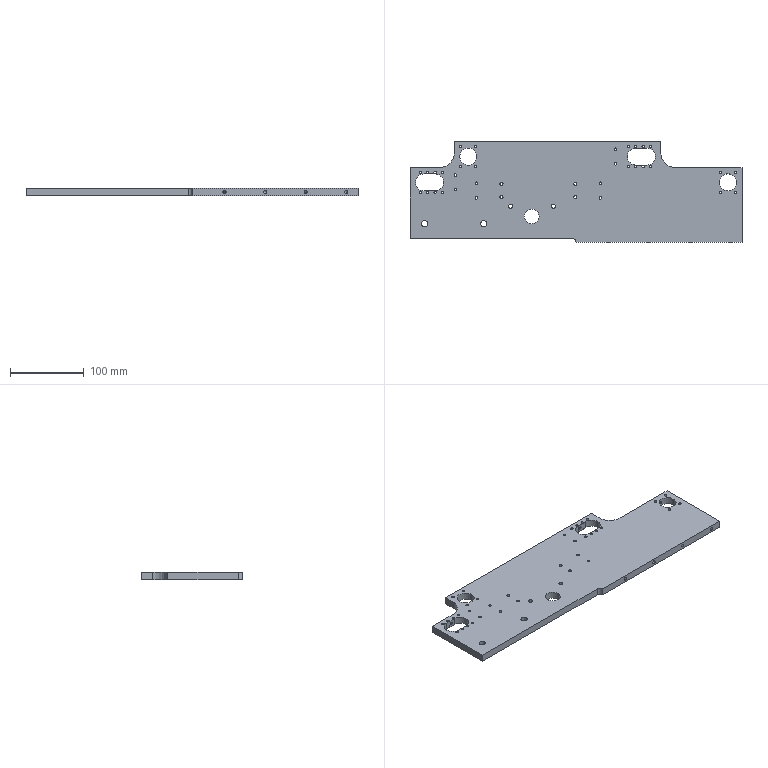Part | STEP file | 08-01 conveyor left baffle | 1 solid | 146 faces | box 450 x 136 x 10 mm | volume 510028 mm3 | cylinder 117 | plane 15 | cone 14 | commonest cylinder face diameters 3.3 x71 4.2 x23 23 x10 5.5 x4 8.5 x4 20 x2